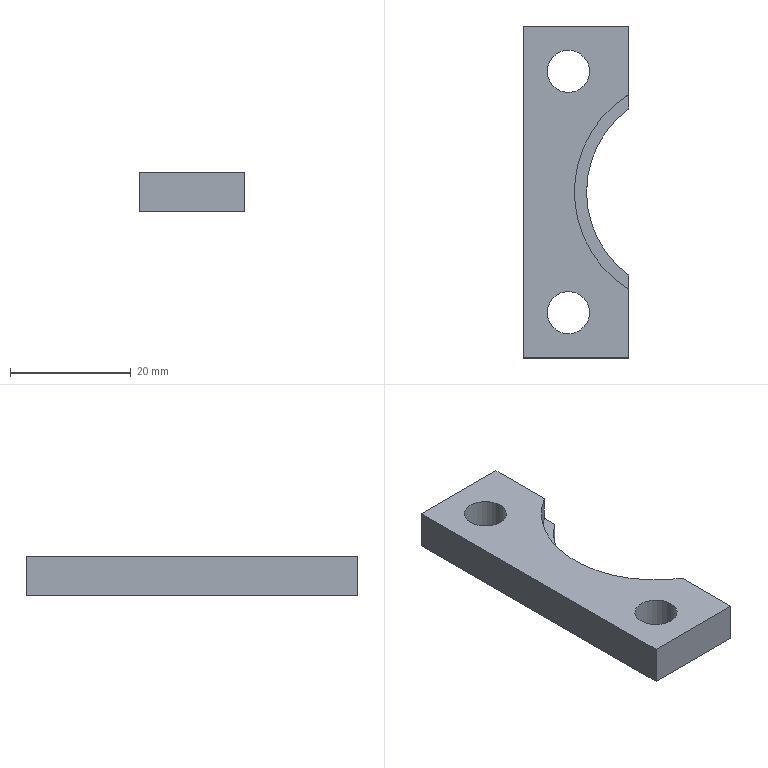Part | NX | features solid 2 | 1 solid | 12 faces | box 17.5 x 55 x 6.5 mm | volume 4597 mm3 | plane 8 | cylinder 4 | commonest cylinder face diameters 7 x2 34 x1 38 x1
STEP:
#1=CARTESIAN_POINT('',(485.5,-267.,395.));
#2=VERTEX_POINT('',#1);
#3=CARTESIAN_POINT('',(482.,-267.,395.));
#4=DIRECTION('',(0.,0.,1.));
#5=DIRECTION('',(1.,0.,0.));
#6=AXIS2_PLACEMENT_3D('',#3,#4,#5);
#7=CIRCLE('',#6,3.5);
#8=EDGE_CURVE('',#2,#2,#7,.F.);
#9=ORIENTED_EDGE('',*,*,#8,.T.);
#10=EDGE_LOOP('',(#9));
#11=FACE_BOUND('',#10,.T.);
#12=CARTESIAN_POINT('',(485.5,-307.,395.));
#13=VERTEX_POINT('',#12);
#14=CARTESIAN_POINT('',(482.,-307.,395.));
#15=DIRECTION('',(0.,0.,1.));
#16=DIRECTION('',(1.,0.,0.));
#17=AXIS2_PLACEMENT_3D('',#14,#15,#16);
#18=CIRCLE('',#17,3.5);
#19=EDGE_CURVE('',#13,#13,#18,.F.);
#20=ORIENTED_EDGE('',*,*,#19,.T.);
#21=EDGE_LOOP('',(#20));
#22=FACE_BOUND('',#21,.T.);
#23=CARTESIAN_POINT('',(492.,-270.845,395.));
#24=VERTEX_POINT('',#23);
#25=CARTESIAN_POINT('',(492.,-303.155,395.));
#26=VERTEX_POINT('',#25);
#27=CARTESIAN_POINT('',(502.,-287.,395.));
#28=DIRECTION('',(0.,0.,1.));
#29=DIRECTION('',(1.,0.,0.));
#30=AXIS2_PLACEMENT_3D('',#27,#28,#29);
#31=CIRCLE('',#30,19.);
#32=EDGE_CURVE('',#24,#26,#31,.T.);
#33=ORIENTED_EDGE('',*,*,#32,.F.);
#34=CARTESIAN_POINT('',(492.,-259.5,395.));
#35=VERTEX_POINT('',#34);
#36=CARTESIAN_POINT('',(492.,-152.,395.));
#37=DIRECTION('',(0.,1.,0.));
#38=VECTOR('',#37,1000.);
#39=LINE('',#36,#38);
#40=EDGE_CURVE('',#35,#24,#39,.F.);
#41=ORIENTED_EDGE('',*,*,#40,.F.);
#42=CARTESIAN_POINT('',(474.5,-259.5,395.));
#43=VERTEX_POINT('',#42);
#44=CARTESIAN_POINT('',(287.,-259.5,395.));
#45=DIRECTION('',(1.,0.,0.));
#46=VECTOR('',#45,1000.);
#47=LINE('',#44,#46);
#48=EDGE_CURVE('',#35,#43,#47,.F.);
#49=ORIENTED_EDGE('',*,*,#48,.T.);
#50=CARTESIAN_POINT('',(474.5,-314.5,395.));
#51=VERTEX_POINT('',#50);
#52=CARTESIAN_POINT('',(474.5,-152.,395.));
#53=DIRECTION('',(0.,1.,0.));
#54=VECTOR('',#53,1000.);
#55=LINE('',#52,#54);
#56=EDGE_CURVE('',#43,#51,#55,.F.);
#57=ORIENTED_EDGE('',*,*,#56,.T.);
#58=CARTESIAN_POINT('',(492.,-314.5,395.));
#59=VERTEX_POINT('',#58);
#60=CARTESIAN_POINT('',(287.,-314.5,395.));
#61=DIRECTION('',(1.,0.,0.));
#62=VECTOR('',#61,1000.);
#63=LINE('',#60,#62);
#64=EDGE_CURVE('',#59,#51,#63,.F.);
#65=ORIENTED_EDGE('',*,*,#64,.F.);
#66=CARTESIAN_POINT('',(492.,-152.,395.));
#67=DIRECTION('',(0.,1.,0.));
#68=VECTOR('',#67,1000.);
#69=LINE('',#66,#68);
#70=EDGE_CURVE('',#26,#59,#69,.F.);
#71=ORIENTED_EDGE('',*,*,#70,.F.);
#72=EDGE_LOOP('',(#33,#41,#49,#57,#65,#71));
#73=FACE_BOUND('',#72,.T.);
#74=CARTESIAN_POINT('',(287.,-152.,395.));
#75=DIRECTION('',(0.,0.,1.));
#76=DIRECTION('',(1.,0.,0.));
#77=AXIS2_PLACEMENT_3D('',#74,#75,#76);
#78=PLANE('',#77);
#79=ADVANCED_FACE('',(#11,#22,#73),#78,.T.);
#80=CARTESIAN_POINT('',(492.,-300.748,391.));
#81=VERTEX_POINT('',#80);
#82=CARTESIAN_POINT('',(492.,-300.748,388.5));
#83=VERTEX_POINT('',#82);
#84=CARTESIAN_POINT('',(492.,-300.748,387.));
#85=DIRECTION('',(0.,0.,1.));
#86=VECTOR('',#85,1000.);
#87=LINE('',#84,#86);
#88=EDGE_CURVE('',#81,#83,#87,.F.);
#89=ORIENTED_EDGE('',*,*,#88,.F.);
#90=CARTESIAN_POINT('',(492.,-303.155,391.));
#91=VERTEX_POINT('',#90);
#92=CARTESIAN_POINT('',(492.,-252.,391.));
#93=DIRECTION('',(0.,1.,0.));
#94=VECTOR('',#93,1000.);
#95=LINE('',#92,#94);
#96=EDGE_CURVE('',#81,#91,#95,.F.);
#97=ORIENTED_EDGE('',*,*,#96,.T.);
#98=CARTESIAN_POINT('',(492.,-303.155,406.));
#99=DIRECTION('',(0.,0.,-1.));
#100=VECTOR('',#99,1000.);
#101=LINE('',#98,#100);
#102=EDGE_CURVE('',#91,#26,#101,.F.);
#103=ORIENTED_EDGE('',*,*,#102,.T.);
#104=ORIENTED_EDGE('',*,*,#70,.T.);
#105=CARTESIAN_POINT('',(492.,-314.5,388.5));
#106=VERTEX_POINT('',#105);
#107=CARTESIAN_POINT('',(492.,-314.5,388.5));
#108=DIRECTION('',(0.,0.,-1.));
#109=VECTOR('',#108,1000.);
#110=LINE('',#107,#109);
#111=EDGE_CURVE('',#59,#106,#110,.T.);
#112=ORIENTED_EDGE('',*,*,#111,.T.);
#113=CARTESIAN_POINT('',(492.,-152.,388.5));
#114=DIRECTION('',(0.,1.,0.));
#115=VECTOR('',#114,1000.);
#116=LINE('',#113,#115);
#117=EDGE_CURVE('',#83,#106,#116,.F.);
#118=ORIENTED_EDGE('',*,*,#117,.F.);
#119=EDGE_LOOP('',(#89,#97,#103,#104,#112,#118));
#120=FACE_BOUND('',#119,.T.);
#121=CARTESIAN_POINT('',(492.,-252.,388.5));
#122=DIRECTION('',(1.,0.,0.));
#123=DIRECTION('',(0.,0.,1.));
#124=AXIS2_PLACEMENT_3D('',#121,#122,#123);
#125=PLANE('',#124);
#126=ADVANCED_FACE('',(#120),#125,.T.);
#127=ORIENTED_EDGE('',*,*,#64,.T.);
#128=CARTESIAN_POINT('',(474.5,-314.5,388.5));
#129=VERTEX_POINT('',#128);
#130=CARTESIAN_POINT('',(474.5,-314.5,388.5));
#131=DIRECTION('',(0.,0.,-1.));
#132=VECTOR('',#131,1000.);
#133=LINE('',#130,#132);
#134=EDGE_CURVE('',#51,#129,#133,.T.);
#135=ORIENTED_EDGE('',*,*,#134,.T.);
#136=CARTESIAN_POINT('',(287.,-314.5,388.5));
#137=DIRECTION('',(1.,0.,0.));
#138=VECTOR('',#137,1000.);
#139=LINE('',#136,#138);
#140=EDGE_CURVE('',#106,#129,#139,.F.);
#141=ORIENTED_EDGE('',*,*,#140,.F.);
#142=ORIENTED_EDGE('',*,*,#111,.F.);
#143=EDGE_LOOP('',(#127,#135,#141,#142));
#144=FACE_BOUND('',#143,.T.);
#145=CARTESIAN_POINT('',(287.,-314.5,388.5));
#146=DIRECTION('',(0.,1.,0.));
#147=DIRECTION('',(0.,0.,-1.));
#148=AXIS2_PLACEMENT_3D('',#145,#146,#147);
#149=PLANE('',#148);
#150=ADVANCED_FACE('',(#144),#149,.F.);
#151=CARTESIAN_POINT('',(492.,-259.5,388.5));
#152=VERTEX_POINT('',#151);
#153=CARTESIAN_POINT('',(474.5,-259.5,388.5));
#154=VERTEX_POINT('',#153);
#155=CARTESIAN_POINT('',(287.,-259.5,388.5));
#156=DIRECTION('',(1.,0.,0.));
#157=VECTOR('',#156,1000.);
#158=LINE('',#155,#157);
#159=EDGE_CURVE('',#152,#154,#158,.F.);
#160=ORIENTED_EDGE('',*,*,#159,.T.);
#161=CARTESIAN_POINT('',(474.5,-259.5,388.5));
#162=DIRECTION('',(0.,0.,1.));
#163=VECTOR('',#162,1000.);
#164=LINE('',#161,#163);
#165=EDGE_CURVE('',#154,#43,#164,.T.);
#166=ORIENTED_EDGE('',*,*,#165,.T.);
#167=ORIENTED_EDGE('',*,*,#48,.F.);
#168=CARTESIAN_POINT('',(492.,-259.5,388.5));
#169=DIRECTION('',(0.,0.,-1.));
#170=VECTOR('',#169,1000.);
#171=LINE('',#168,#170);
#172=EDGE_CURVE('',#35,#152,#171,.T.);
#173=ORIENTED_EDGE('',*,*,#172,.T.);
#174=EDGE_LOOP('',(#160,#166,#167,#173));
#175=FACE_BOUND('',#174,.T.);
#176=CARTESIAN_POINT('',(287.,-259.5,388.5));
#177=DIRECTION('',(0.,1.,0.));
#178=DIRECTION('',(-1.,0.,0.));
#179=AXIS2_PLACEMENT_3D('',#176,#177,#178);
#180=PLANE('',#179);
#181=ADVANCED_FACE('',(#175),#180,.T.);
#182=CARTESIAN_POINT('',(492.,-273.252,388.5));
#183=VERTEX_POINT('',#182);
#184=CARTESIAN_POINT('',(502.,-287.,388.5));
#185=DIRECTION('',(0.,0.,1.));
#186=DIRECTION('',(1.,0.,0.));
#187=AXIS2_PLACEMENT_3D('',#184,#185,#186);
#188=CIRCLE('',#187,17.);
#189=EDGE_CURVE('',#83,#183,#188,.F.);
#190=ORIENTED_EDGE('',*,*,#189,.F.);
#191=ORIENTED_EDGE('',*,*,#117,.T.);
#192=ORIENTED_EDGE('',*,*,#140,.T.);
#193=CARTESIAN_POINT('',(474.5,-152.,388.5));
#194=DIRECTION('',(0.,1.,0.));
#195=VECTOR('',#194,1000.);
#196=LINE('',#193,#195);
#197=EDGE_CURVE('',#154,#129,#196,.F.);
#198=ORIENTED_EDGE('',*,*,#197,.F.);
#199=ORIENTED_EDGE('',*,*,#159,.F.);
#200=CARTESIAN_POINT('',(492.,-152.,388.5));
#201=DIRECTION('',(0.,1.,0.));
#202=VECTOR('',#201,1000.);
#203=LINE('',#200,#202);
#204=EDGE_CURVE('',#152,#183,#203,.F.);
#205=ORIENTED_EDGE('',*,*,#204,.T.);
#206=EDGE_LOOP('',(#190,#191,#192,#198,#199,#205));
#207=FACE_BOUND('',#206,.T.);
#208=CARTESIAN_POINT('',(485.5,-307.,388.5));
#209=VERTEX_POINT('',#208);
#210=CARTESIAN_POINT('',(482.,-307.,388.5));
#211=DIRECTION('',(0.,0.,1.));
#212=DIRECTION('',(1.,0.,0.));
#213=AXIS2_PLACEMENT_3D('',#210,#211,#212);
#214=CIRCLE('',#213,3.5);
#215=EDGE_CURVE('',#209,#209,#214,.T.);
#216=ORIENTED_EDGE('',*,*,#215,.T.);
#217=EDGE_LOOP('',(#216));
#218=FACE_BOUND('',#217,.T.);
#219=CARTESIAN_POINT('',(485.5,-267.,388.5));
#220=VERTEX_POINT('',#219);
#221=CARTESIAN_POINT('',(482.,-267.,388.5));
#222=DIRECTION('',(0.,0.,1.));
#223=DIRECTION('',(1.,0.,0.));
#224=AXIS2_PLACEMENT_3D('',#221,#222,#223);
#225=CIRCLE('',#224,3.5);
#226=EDGE_CURVE('',#220,#220,#225,.T.);
#227=ORIENTED_EDGE('',*,*,#226,.T.);
#228=EDGE_LOOP('',(#227));
#229=FACE_BOUND('',#228,.T.);
#230=CARTESIAN_POINT('',(287.,-152.,388.5));
#231=DIRECTION('',(0.,0.,1.));
#232=DIRECTION('',(1.,0.,0.));
#233=AXIS2_PLACEMENT_3D('',#230,#231,#232);
#234=PLANE('',#233);
#235=ADVANCED_FACE('',(#207,#218,#229),#234,.F.);
#236=ORIENTED_EDGE('',*,*,#197,.T.);
#237=ORIENTED_EDGE('',*,*,#134,.F.);
#238=ORIENTED_EDGE('',*,*,#56,.F.);
#239=ORIENTED_EDGE('',*,*,#165,.F.);
#240=EDGE_LOOP('',(#236,#237,#238,#239));
#241=FACE_BOUND('',#240,.T.);
#242=CARTESIAN_POINT('',(474.5,-152.,388.5));
#243=DIRECTION('',(-1.,0.,0.));
#244=DIRECTION('',(0.,0.,-1.));
#245=AXIS2_PLACEMENT_3D('',#242,#243,#244);
#246=PLANE('',#245);
#247=ADVANCED_FACE('',(#241),#246,.T.);
#248=CARTESIAN_POINT('',(492.,-273.252,391.));
#249=VERTEX_POINT('',#248);
#250=CARTESIAN_POINT('',(492.,-273.252,387.));
#251=DIRECTION('',(0.,0.,1.));
#252=VECTOR('',#251,1000.);
#253=LINE('',#250,#252);
#254=EDGE_CURVE('',#183,#249,#253,.T.);
#255=ORIENTED_EDGE('',*,*,#254,.F.);
#256=ORIENTED_EDGE('',*,*,#204,.F.);
#257=ORIENTED_EDGE('',*,*,#172,.F.);
#258=ORIENTED_EDGE('',*,*,#40,.T.);
#259=CARTESIAN_POINT('',(492.,-270.845,391.));
#260=VERTEX_POINT('',#259);
#261=CARTESIAN_POINT('',(492.,-270.845,406.));
#262=DIRECTION('',(0.,0.,-1.));
#263=VECTOR('',#262,1000.);
#264=LINE('',#261,#263);
#265=EDGE_CURVE('',#24,#260,#264,.T.);
#266=ORIENTED_EDGE('',*,*,#265,.T.);
#267=CARTESIAN_POINT('',(492.,-252.,391.));
#268=DIRECTION('',(0.,1.,0.));
#269=VECTOR('',#268,1000.);
#270=LINE('',#267,#269);
#271=EDGE_CURVE('',#260,#249,#270,.F.);
#272=ORIENTED_EDGE('',*,*,#271,.T.);
#273=EDGE_LOOP('',(#255,#256,#257,#258,#266,#272));
#274=FACE_BOUND('',#273,.T.);
#275=CARTESIAN_POINT('',(492.,-252.,388.5));
#276=DIRECTION('',(1.,0.,0.));
#277=DIRECTION('',(0.,0.,1.));
#278=AXIS2_PLACEMENT_3D('',#275,#276,#277);
#279=PLANE('',#278);
#280=ADVANCED_FACE('',(#274),#279,.T.);
#281=ORIENTED_EDGE('',*,*,#226,.F.);
#282=EDGE_LOOP('',(#281));
#283=FACE_BOUND('',#282,.T.);
#284=ORIENTED_EDGE('',*,*,#8,.F.);
#285=EDGE_LOOP('',(#284));
#286=FACE_BOUND('',#285,.T.);
#287=CARTESIAN_POINT('',(482.,-267.,388.5));
#288=DIRECTION('',(0.,0.,1.));
#289=DIRECTION('',(1.,0.,0.));
#290=AXIS2_PLACEMENT_3D('',#287,#288,#289);
#291=CYLINDRICAL_SURFACE('',#290,3.5);
#292=ADVANCED_FACE('',(#283,#286),#291,.F.);
#293=ORIENTED_EDGE('',*,*,#215,.F.);
#294=EDGE_LOOP('',(#293));
#295=FACE_BOUND('',#294,.T.);
#296=ORIENTED_EDGE('',*,*,#19,.F.);
#297=EDGE_LOOP('',(#296));
#298=FACE_BOUND('',#297,.T.);
#299=CARTESIAN_POINT('',(482.,-307.,388.5));
#300=DIRECTION('',(0.,0.,1.));
#301=DIRECTION('',(1.,0.,0.));
#302=AXIS2_PLACEMENT_3D('',#299,#300,#301);
#303=CYLINDRICAL_SURFACE('',#302,3.5);
#304=ADVANCED_FACE('',(#295,#298),#303,.F.);
#305=ORIENTED_EDGE('',*,*,#254,.T.);
#306=CARTESIAN_POINT('',(502.,-287.,391.));
#307=DIRECTION('',(0.,0.,1.));
#308=DIRECTION('',(1.,0.,0.));
#309=AXIS2_PLACEMENT_3D('',#306,#307,#308);
#310=CIRCLE('',#309,17.);
#311=EDGE_CURVE('',#249,#81,#310,.T.);
#312=ORIENTED_EDGE('',*,*,#311,.T.);
#313=ORIENTED_EDGE('',*,*,#88,.T.);
#314=ORIENTED_EDGE('',*,*,#189,.T.);
#315=EDGE_LOOP('',(#305,#312,#313,#314));
#316=FACE_BOUND('',#315,.T.);
#317=CARTESIAN_POINT('',(502.,-287.,387.));
#318=DIRECTION('',(0.,0.,1.));
#319=DIRECTION('',(1.,0.,0.));
#320=AXIS2_PLACEMENT_3D('',#317,#318,#319);
#321=CYLINDRICAL_SURFACE('',#320,17.);
#322=ADVANCED_FACE('',(#316),#321,.F.);
#323=CARTESIAN_POINT('',(502.,-287.,391.));
#324=DIRECTION('',(0.,0.,1.));
#325=DIRECTION('',(1.,0.,0.));
#326=AXIS2_PLACEMENT_3D('',#323,#324,#325);
#327=CIRCLE('',#326,19.);
#328=EDGE_CURVE('',#260,#91,#327,.T.);
#329=ORIENTED_EDGE('',*,*,#328,.T.);
#330=ORIENTED_EDGE('',*,*,#96,.F.);
#331=ORIENTED_EDGE('',*,*,#311,.F.);
#332=ORIENTED_EDGE('',*,*,#271,.F.);
#333=EDGE_LOOP('',(#329,#330,#331,#332));
#334=FACE_BOUND('',#333,.T.);
#335=CARTESIAN_POINT('',(502.,-287.,391.));
#336=DIRECTION('',(0.,0.,-1.));
#337=DIRECTION('',(-1.,0.,0.));
#338=AXIS2_PLACEMENT_3D('',#335,#336,#337);
#339=PLANE('',#338);
#340=ADVANCED_FACE('',(#334),#339,.F.);
#341=ORIENTED_EDGE('',*,*,#328,.F.);
#342=ORIENTED_EDGE('',*,*,#265,.F.);
#343=ORIENTED_EDGE('',*,*,#32,.T.);
#344=ORIENTED_EDGE('',*,*,#102,.F.);
#345=EDGE_LOOP('',(#341,#342,#343,#344));
#346=FACE_BOUND('',#345,.T.);
#347=CARTESIAN_POINT('',(502.,-287.,406.));
#348=DIRECTION('',(0.,0.,-1.));
#349=DIRECTION('',(-1.,0.,0.));
#350=AXIS2_PLACEMENT_3D('',#347,#348,#349);
#351=CYLINDRICAL_SURFACE('',#350,19.);
#352=ADVANCED_FACE('',(#346),#351,.F.);
#353=CLOSED_SHELL('',(#79,#126,#150,#181,#235,#247,#280,#292,#304,#322,#340,#352));
#354=MANIFOLD_SOLID_BREP('',#353);
#355=(LENGTH_UNIT()NAMED_UNIT(*)SI_UNIT(.MILLI.,.METRE.));
#356=UNCERTAINTY_MEASURE_WITH_UNIT(LENGTH_MEASURE(0.00001),#355,'','');
#357=(NAMED_UNIT(*)PLANE_ANGLE_UNIT()SI_UNIT($,.RADIAN.));
#358=(NAMED_UNIT(*)SI_UNIT($,.STERADIAN.)SOLID_ANGLE_UNIT());
#359=(GEOMETRIC_REPRESENTATION_CONTEXT(3)GLOBAL_UNCERTAINTY_ASSIGNED_CONTEXT((#356))GLOBAL_UNIT_ASSIGNED_CONTEXT((#355,#357,#358))REPRESENTATION_CONTEXT('',''));
#360=ADVANCED_BREP_SHAPE_REPRESENTATION('',(#354),#359);